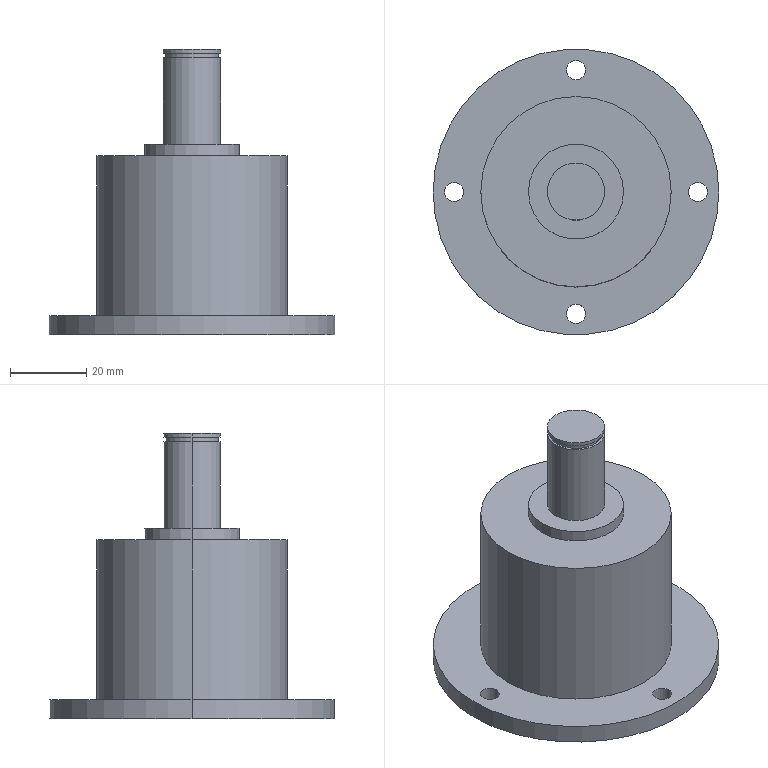Part | STEP file | Push-film driven bearing seat SGN-3-04 | 1 solid | 27 faces | box 75 x 75 x 75 mm | volume 110021 mm3 | cylinder 20 | plane 7 | commonest cylinder face diameters 5 x8 15 x4 13.8 x2 25 x2 50 x2 75 x2